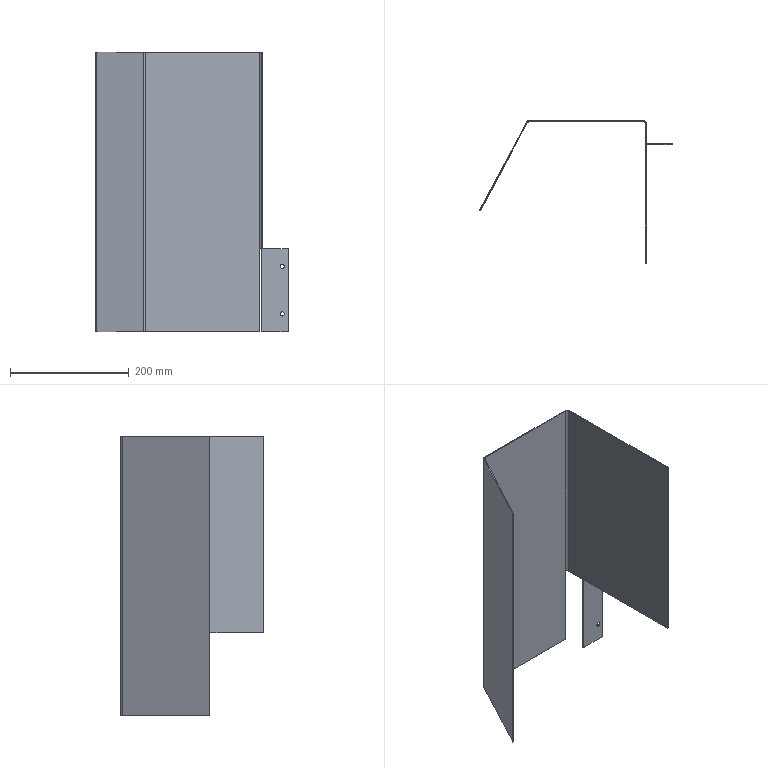Part | SolidWorks | features ICE 4, Extrusion 1, MoveFace 1 | 1 solid | 26 faces | box 323.5 x 240 x 470 mm | volume 385016 mm3 | plane 18 | cylinder 8 | commonest cylinder face diameters 7 x6 10 x2
STEP:
#1=CARTESIAN_POINT('',(313.5,110.,26.5));
#2=VERTEX_POINT('',#1);
#3=CARTESIAN_POINT('',(313.5,110.,33.5));
#4=VERTEX_POINT('',#3);
#5=CARTESIAN_POINT('',(313.5,110.,30.));
#6=DIRECTION('',(0.,1.,0.));
#7=DIRECTION('',(0.,0.,1.));
#8=AXIS2_PLACEMENT_3D('',#5,#6,#7);
#9=CIRCLE('',#8,3.5);
#10=EDGE_CURVE('',#2,#4,#9,.T.);
#11=ORIENTED_EDGE('',*,*,#10,.F.);
#12=CARTESIAN_POINT('',(313.5,111.5,26.5));
#13=VERTEX_POINT('',#12);
#14=CARTESIAN_POINT('',(313.5,110.,26.5));
#15=DIRECTION('',(0.,1.,0.));
#16=VECTOR('',#15,1000.);
#17=LINE('',#14,#16);
#18=EDGE_CURVE('',#2,#13,#17,.T.);
#19=ORIENTED_EDGE('',*,*,#18,.T.);
#20=CARTESIAN_POINT('',(313.5,111.5,33.5));
#21=VERTEX_POINT('',#20);
#22=CARTESIAN_POINT('',(313.5,111.5,30.));
#23=DIRECTION('',(0.,1.,0.));
#24=DIRECTION('',(0.,0.,1.));
#25=AXIS2_PLACEMENT_3D('',#22,#23,#24);
#26=CIRCLE('',#25,3.5);
#27=EDGE_CURVE('',#13,#21,#26,.T.);
#28=ORIENTED_EDGE('',*,*,#27,.T.);
#29=CARTESIAN_POINT('',(313.5,110.,33.5));
#30=DIRECTION('',(0.,1.,0.));
#31=VECTOR('',#30,1000.);
#32=LINE('',#29,#31);
#33=EDGE_CURVE('',#4,#21,#32,.T.);
#34=ORIENTED_EDGE('',*,*,#33,.F.);
#35=EDGE_LOOP('',(#11,#19,#28,#34));
#36=FACE_OUTER_BOUND('',#35,.T.);
#37=CARTESIAN_POINT('',(313.5,110.,30.));
#38=DIRECTION('',(0.,1.,0.));
#39=DIRECTION('',(0.,0.,1.));
#40=AXIS2_PLACEMENT_3D('',#37,#38,#39);
#41=CYLINDRICAL_SURFACE('',#40,3.5);
#42=ADVANCED_FACE('',(#36),#41,.F.);
#43=CARTESIAN_POINT('',(313.5,110.,106.5));
#44=VERTEX_POINT('',#43);
#45=CARTESIAN_POINT('',(313.5,110.,113.5));
#46=VERTEX_POINT('',#45);
#47=CARTESIAN_POINT('',(313.5,110.,110.));
#48=DIRECTION('',(0.,1.,0.));
#49=DIRECTION('',(0.,0.,1.));
#50=AXIS2_PLACEMENT_3D('',#47,#48,#49);
#51=CIRCLE('',#50,3.5);
#52=EDGE_CURVE('',#44,#46,#51,.T.);
#53=ORIENTED_EDGE('',*,*,#52,.F.);
#54=CARTESIAN_POINT('',(313.5,111.5,106.5));
#55=VERTEX_POINT('',#54);
#56=CARTESIAN_POINT('',(313.5,110.,106.5));
#57=DIRECTION('',(0.,1.,0.));
#58=VECTOR('',#57,1000.);
#59=LINE('',#56,#58);
#60=EDGE_CURVE('',#44,#55,#59,.T.);
#61=ORIENTED_EDGE('',*,*,#60,.T.);
#62=CARTESIAN_POINT('',(313.5,111.5,113.5));
#63=VERTEX_POINT('',#62);
#64=CARTESIAN_POINT('',(313.5,111.5,110.));
#65=DIRECTION('',(0.,1.,0.));
#66=DIRECTION('',(0.,0.,1.));
#67=AXIS2_PLACEMENT_3D('',#64,#65,#66);
#68=CIRCLE('',#67,3.5);
#69=EDGE_CURVE('',#55,#63,#68,.T.);
#70=ORIENTED_EDGE('',*,*,#69,.T.);
#71=CARTESIAN_POINT('',(313.5,110.,113.5));
#72=DIRECTION('',(0.,1.,0.));
#73=VECTOR('',#72,1000.);
#74=LINE('',#71,#73);
#75=EDGE_CURVE('',#46,#63,#74,.T.);
#76=ORIENTED_EDGE('',*,*,#75,.F.);
#77=EDGE_LOOP('',(#53,#61,#70,#76));
#78=FACE_OUTER_BOUND('',#77,.T.);
#79=CARTESIAN_POINT('',(313.5,110.,110.));
#80=DIRECTION('',(0.,1.,0.));
#81=DIRECTION('',(0.,0.,1.));
#82=AXIS2_PLACEMENT_3D('',#79,#80,#81);
#83=CYLINDRICAL_SURFACE('',#82,3.5);
#84=ADVANCED_FACE('',(#78),#83,.F.);
#85=CARTESIAN_POINT('',(278.5,110.,140.));
#86=VERTEX_POINT('',#85);
#87=CARTESIAN_POINT('',(278.5,-90.,140.));
#88=VERTEX_POINT('',#87);
#89=CARTESIAN_POINT('',(278.5,145.,140.));
#90=DIRECTION('',(0.,-1.,0.));
#91=VECTOR('',#90,1000.);
#92=LINE('',#89,#91);
#93=EDGE_CURVE('',#86,#88,#92,.T.);
#94=ORIENTED_EDGE('',*,*,#93,.F.);
#95=CARTESIAN_POINT('',(280.,110.,140.));
#96=VERTEX_POINT('',#95);
#97=CARTESIAN_POINT('',(280.,110.,140.));
#98=DIRECTION('',(1.,0.,0.));
#99=VECTOR('',#98,1000.);
#100=LINE('',#97,#99);
#101=EDGE_CURVE('',#86,#96,#100,.T.);
#102=ORIENTED_EDGE('',*,*,#101,.T.);
#103=CARTESIAN_POINT('',(280.,-90.,140.));
#104=VERTEX_POINT('',#103);
#105=CARTESIAN_POINT('',(280.,145.,140.));
#106=DIRECTION('',(0.,-1.,0.));
#107=VECTOR('',#106,1000.);
#108=LINE('',#105,#107);
#109=EDGE_CURVE('',#96,#104,#108,.T.);
#110=ORIENTED_EDGE('',*,*,#109,.T.);
#111=CARTESIAN_POINT('',(280.,-90.,140.));
#112=DIRECTION('',(1.,0.,0.));
#113=VECTOR('',#112,1000.);
#114=LINE('',#111,#113);
#115=EDGE_CURVE('',#88,#104,#114,.T.);
#116=ORIENTED_EDGE('',*,*,#115,.F.);
#117=EDGE_LOOP('',(#94,#102,#110,#116));
#118=FACE_OUTER_BOUND('',#117,.T.);
#119=CARTESIAN_POINT('',(280.,145.,140.));
#120=DIRECTION('',(0.,0.,-1.));
#121=DIRECTION('',(-1.,0.,0.));
#122=AXIS2_PLACEMENT_3D('',#119,#120,#121);
#123=PLANE('',#122);
#124=ADVANCED_FACE('',(#118),#123,.T.);
#125=CARTESIAN_POINT('',(278.5,145.,140.));
#126=VERTEX_POINT('',#125);
#127=CARTESIAN_POINT('',(278.5,111.5,140.));
#128=VERTEX_POINT('',#127);
#129=CARTESIAN_POINT('',(278.5,145.,140.));
#130=DIRECTION('',(0.,-1.,0.));
#131=VECTOR('',#130,1000.);
#132=LINE('',#129,#131);
#133=EDGE_CURVE('',#126,#128,#132,.T.);
#134=ORIENTED_EDGE('',*,*,#133,.T.);
#135=CARTESIAN_POINT('',(278.5,111.5,0.));
#136=VERTEX_POINT('',#135);
#137=CARTESIAN_POINT('',(278.5,111.5,0.));
#138=DIRECTION('',(0.,0.,1.));
#139=VECTOR('',#138,1000.);
#140=LINE('',#137,#139);
#141=EDGE_CURVE('',#136,#128,#140,.T.);
#142=ORIENTED_EDGE('',*,*,#141,.F.);
#143=CARTESIAN_POINT('',(278.5,110.,0.));
#144=VERTEX_POINT('',#143);
#145=CARTESIAN_POINT('',(278.5,111.5,0.));
#146=DIRECTION('',(0.,-1.,0.));
#147=VECTOR('',#146,1000.);
#148=LINE('',#145,#147);
#149=EDGE_CURVE('',#136,#144,#148,.T.);
#150=ORIENTED_EDGE('',*,*,#149,.T.);
#151=CARTESIAN_POINT('',(278.5,110.,0.));
#152=DIRECTION('',(0.,0.,1.));
#153=VECTOR('',#152,1000.);
#154=LINE('',#151,#153);
#155=EDGE_CURVE('',#144,#86,#154,.T.);
#156=ORIENTED_EDGE('',*,*,#155,.T.);
#157=ORIENTED_EDGE('',*,*,#93,.T.);
#158=CARTESIAN_POINT('',(278.5,-90.,470.));
#159=VERTEX_POINT('',#158);
#160=CARTESIAN_POINT('',(278.5,-90.,470.));
#161=DIRECTION('',(0.,0.,-1.));
#162=VECTOR('',#161,1000.);
#163=LINE('',#160,#162);
#164=EDGE_CURVE('',#159,#88,#163,.T.);
#165=ORIENTED_EDGE('',*,*,#164,.F.);
#166=CARTESIAN_POINT('',(278.5,145.,470.));
#167=VERTEX_POINT('',#166);
#168=CARTESIAN_POINT('',(278.5,145.,470.));
#169=DIRECTION('',(0.,-1.,0.));
#170=VECTOR('',#169,1000.);
#171=LINE('',#168,#170);
#172=EDGE_CURVE('',#167,#159,#171,.T.);
#173=ORIENTED_EDGE('',*,*,#172,.F.);
#174=CARTESIAN_POINT('',(278.5,145.,470.));
#175=DIRECTION('',(0.,0.,-1.));
#176=VECTOR('',#175,1000.);
#177=LINE('',#174,#176);
#178=EDGE_CURVE('',#167,#126,#177,.T.);
#179=ORIENTED_EDGE('',*,*,#178,.T.);
#180=EDGE_LOOP('',(#134,#142,#150,#156,#157,#165,#173,#179));
#181=FACE_OUTER_BOUND('',#180,.T.);
#182=CARTESIAN_POINT('',(278.5,145.,470.));
#183=DIRECTION('',(1.,0.,0.));
#184=DIRECTION('',(0.,1.,0.));
#185=AXIS2_PLACEMENT_3D('',#182,#183,#184);
#186=PLANE('',#185);
#187=ADVANCED_FACE('',(#181),#186,.F.);
#188=ORIENTED_EDGE('',*,*,#164,.T.);
#189=ORIENTED_EDGE('',*,*,#115,.T.);
#190=CARTESIAN_POINT('',(280.,-90.,470.));
#191=VERTEX_POINT('',#190);
#192=CARTESIAN_POINT('',(280.,-90.,470.));
#193=DIRECTION('',(0.,0.,-1.));
#194=VECTOR('',#193,1000.);
#195=LINE('',#192,#194);
#196=EDGE_CURVE('',#191,#104,#195,.T.);
#197=ORIENTED_EDGE('',*,*,#196,.F.);
#198=CARTESIAN_POINT('',(280.,-90.,470.));
#199=DIRECTION('',(-1.,0.,0.));
#200=VECTOR('',#199,1000.);
#201=LINE('',#198,#200);
#202=EDGE_CURVE('',#191,#159,#201,.T.);
#203=ORIENTED_EDGE('',*,*,#202,.T.);
#204=EDGE_LOOP('',(#188,#189,#197,#203));
#205=FACE_OUTER_BOUND('',#204,.T.);
#206=CARTESIAN_POINT('',(280.,-90.,470.));
#207=DIRECTION('',(0.,-1.,0.));
#208=DIRECTION('',(0.,0.,-1.));
#209=AXIS2_PLACEMENT_3D('',#206,#207,#208);
#210=PLANE('',#209);
#211=ADVANCED_FACE('',(#205),#210,.T.);
#212=ORIENTED_EDGE('',*,*,#196,.T.);
#213=ORIENTED_EDGE('',*,*,#109,.F.);
#214=CARTESIAN_POINT('',(280.,111.5,140.));
#215=VERTEX_POINT('',#214);
#216=CARTESIAN_POINT('',(280.,145.,140.));
#217=DIRECTION('',(0.,-1.,0.));
#218=VECTOR('',#217,1000.);
#219=LINE('',#216,#218);
#220=EDGE_CURVE('',#215,#96,#219,.T.);
#221=ORIENTED_EDGE('',*,*,#220,.F.);
#222=CARTESIAN_POINT('',(280.,145.,140.));
#223=VERTEX_POINT('',#222);
#224=CARTESIAN_POINT('',(280.,145.,140.));
#225=DIRECTION('',(0.,-1.,0.));
#226=VECTOR('',#225,1000.);
#227=LINE('',#224,#226);
#228=EDGE_CURVE('',#223,#215,#227,.T.);
#229=ORIENTED_EDGE('',*,*,#228,.F.);
#230=CARTESIAN_POINT('',(280.,145.,470.));
#231=VERTEX_POINT('',#230);
#232=CARTESIAN_POINT('',(280.,145.,470.));
#233=DIRECTION('',(0.,0.,-1.));
#234=VECTOR('',#233,1000.);
#235=LINE('',#232,#234);
#236=EDGE_CURVE('',#231,#223,#235,.T.);
#237=ORIENTED_EDGE('',*,*,#236,.F.);
#238=CARTESIAN_POINT('',(280.,145.,470.));
#239=DIRECTION('',(0.,-1.,0.));
#240=VECTOR('',#239,1000.);
#241=LINE('',#238,#240);
#242=EDGE_CURVE('',#231,#191,#241,.T.);
#243=ORIENTED_EDGE('',*,*,#242,.T.);
#244=EDGE_LOOP('',(#212,#213,#221,#229,#237,#243));
#245=FACE_OUTER_BOUND('',#244,.T.);
#246=CARTESIAN_POINT('',(280.,145.,470.));
#247=DIRECTION('',(1.,0.,0.));
#248=DIRECTION('',(0.,1.,0.));
#249=AXIS2_PLACEMENT_3D('',#246,#247,#248);
#250=PLANE('',#249);
#251=ADVANCED_FACE('',(#245),#250,.T.);
#252=CARTESIAN_POINT('',(275.,148.5,0.));
#253=VERTEX_POINT('',#252);
#254=CARTESIAN_POINT('',(275.,150.,0.));
#255=VERTEX_POINT('',#254);
#256=CARTESIAN_POINT('',(275.,91.5,0.));
#257=DIRECTION('',(0.,1.,0.));
#258=VECTOR('',#257,1000.);
#259=LINE('',#256,#258);
#260=EDGE_CURVE('',#253,#255,#259,.T.);
#261=ORIENTED_EDGE('',*,*,#260,.F.);
#262=CARTESIAN_POINT('',(83.,148.5,0.));
#263=VERTEX_POINT('',#262);
#264=CARTESIAN_POINT('',(83.,148.5,0.));
#265=DIRECTION('',(1.,0.,0.));
#266=VECTOR('',#265,1000.);
#267=LINE('',#264,#266);
#268=EDGE_CURVE('',#263,#253,#267,.T.);
#269=ORIENTED_EDGE('',*,*,#268,.F.);
#270=CARTESIAN_POINT('',(79.912,146.647,0.));
#271=VERTEX_POINT('',#270);
#272=CARTESIAN_POINT('',(83.,145.,0.));
#273=DIRECTION('',(0.,0.,-1.));
#274=DIRECTION('',(-1.,0.,0.));
#275=AXIS2_PLACEMENT_3D('',#272,#273,#274);
#276=CIRCLE('',#275,3.5);
#277=EDGE_CURVE('',#271,#263,#276,.T.);
#278=ORIENTED_EDGE('',*,*,#277,.F.);
#279=CARTESIAN_POINT('',(1.7,0.,0.));
#280=VERTEX_POINT('',#279);
#281=CARTESIAN_POINT('',(1.7,0.,0.));
#282=DIRECTION('',(0.4706,0.8824,0.));
#283=VECTOR('',#282,1000.);
#284=LINE('',#281,#283);
#285=EDGE_CURVE('',#280,#271,#284,.T.);
#286=ORIENTED_EDGE('',*,*,#285,.F.);
#287=CARTESIAN_POINT('',(0.,0.,0.));
#288=VERTEX_POINT('',#287);
#289=CARTESIAN_POINT('',(0.,0.,0.));
#290=DIRECTION('',(1.,0.,0.));
#291=VECTOR('',#290,1000.);
#292=LINE('',#289,#291);
#293=EDGE_CURVE('',#288,#280,#292,.T.);
#294=ORIENTED_EDGE('',*,*,#293,.F.);
#295=CARTESIAN_POINT('',(78.588,147.353,0.));
#296=VERTEX_POINT('',#295);
#297=CARTESIAN_POINT('',(0.,0.,0.));
#298=DIRECTION('',(0.4706,0.8824,0.));
#299=VECTOR('',#298,1000.);
#300=LINE('',#297,#299);
#301=EDGE_CURVE('',#288,#296,#300,.T.);
#302=ORIENTED_EDGE('',*,*,#301,.T.);
#303=CARTESIAN_POINT('',(83.,150.,0.));
#304=VERTEX_POINT('',#303);
#305=CARTESIAN_POINT('',(83.,145.,0.));
#306=DIRECTION('',(0.,0.,-1.));
#307=DIRECTION('',(-1.,0.,0.));
#308=AXIS2_PLACEMENT_3D('',#305,#306,#307);
#309=CIRCLE('',#308,5.);
#310=EDGE_CURVE('',#296,#304,#309,.T.);
#311=ORIENTED_EDGE('',*,*,#310,.T.);
#312=CARTESIAN_POINT('',(83.,150.,0.));
#313=DIRECTION('',(1.,0.,0.));
#314=VECTOR('',#313,1000.);
#315=LINE('',#312,#314);
#316=EDGE_CURVE('',#304,#255,#315,.T.);
#317=ORIENTED_EDGE('',*,*,#316,.T.);
#318=EDGE_LOOP('',(#261,#269,#278,#286,#294,#302,#311,#317));
#319=FACE_OUTER_BOUND('',#318,.T.);
#320=CARTESIAN_POINT('',(83.,145.,0.));
#321=DIRECTION('',(0.,0.,-1.));
#322=DIRECTION('',(-1.,0.,0.));
#323=AXIS2_PLACEMENT_3D('',#320,#321,#322);
#324=PLANE('',#323);
#325=ADVANCED_FACE('',(#319),#324,.T.);
#326=ORIENTED_EDGE('',*,*,#293,.T.);
#327=CARTESIAN_POINT('',(1.7,0.,470.));
#328=VERTEX_POINT('',#327);
#329=CARTESIAN_POINT('',(1.7,0.,470.));
#330=DIRECTION('',(0.,0.,-1.));
#331=VECTOR('',#330,1000.);
#332=LINE('',#329,#331);
#333=EDGE_CURVE('',#328,#280,#332,.T.);
#334=ORIENTED_EDGE('',*,*,#333,.F.);
#335=CARTESIAN_POINT('',(0.,0.,470.));
#336=VERTEX_POINT('',#335);
#337=CARTESIAN_POINT('',(0.,0.,470.));
#338=DIRECTION('',(1.,0.,0.));
#339=VECTOR('',#338,1000.);
#340=LINE('',#337,#339);
#341=EDGE_CURVE('',#336,#328,#340,.T.);
#342=ORIENTED_EDGE('',*,*,#341,.F.);
#343=CARTESIAN_POINT('',(0.,0.,470.));
#344=DIRECTION('',(0.,0.,-1.));
#345=VECTOR('',#344,1000.);
#346=LINE('',#343,#345);
#347=EDGE_CURVE('',#336,#288,#346,.T.);
#348=ORIENTED_EDGE('',*,*,#347,.T.);
#349=EDGE_LOOP('',(#326,#334,#342,#348));
#350=FACE_OUTER_BOUND('',#349,.T.);
#351=CARTESIAN_POINT('',(0.,0.,470.));
#352=DIRECTION('',(0.,1.,0.));
#353=DIRECTION('',(0.,0.,1.));
#354=AXIS2_PLACEMENT_3D('',#351,#352,#353);
#355=PLANE('',#354);
#356=ADVANCED_FACE('',(#350),#355,.F.);
#357=ORIENTED_EDGE('',*,*,#285,.T.);
#358=CARTESIAN_POINT('',(79.912,146.647,470.));
#359=VERTEX_POINT('',#358);
#360=CARTESIAN_POINT('',(79.912,146.647,470.));
#361=DIRECTION('',(0.,0.,-1.));
#362=VECTOR('',#361,1000.);
#363=LINE('',#360,#362);
#364=EDGE_CURVE('',#359,#271,#363,.T.);
#365=ORIENTED_EDGE('',*,*,#364,.F.);
#366=CARTESIAN_POINT('',(1.7,0.,470.));
#367=DIRECTION('',(0.4706,0.8824,0.));
#368=VECTOR('',#367,1000.);
#369=LINE('',#366,#368);
#370=EDGE_CURVE('',#328,#359,#369,.T.);
#371=ORIENTED_EDGE('',*,*,#370,.F.);
#372=ORIENTED_EDGE('',*,*,#333,.T.);
#373=EDGE_LOOP('',(#357,#365,#371,#372));
#374=FACE_OUTER_BOUND('',#373,.T.);
#375=CARTESIAN_POINT('',(1.7,0.,470.));
#376=DIRECTION('',(-0.8824,0.4706,0.));
#377=DIRECTION('',(-0.4706,-0.8824,0.));
#378=AXIS2_PLACEMENT_3D('',#375,#376,#377);
#379=PLANE('',#378);
#380=ADVANCED_FACE('',(#374),#379,.F.);
#381=ORIENTED_EDGE('',*,*,#277,.T.);
#382=CARTESIAN_POINT('',(83.,148.5,470.));
#383=VERTEX_POINT('',#382);
#384=CARTESIAN_POINT('',(83.,148.5,470.));
#385=DIRECTION('',(0.,0.,-1.));
#386=VECTOR('',#385,1000.);
#387=LINE('',#384,#386);
#388=EDGE_CURVE('',#383,#263,#387,.T.);
#389=ORIENTED_EDGE('',*,*,#388,.F.);
#390=CARTESIAN_POINT('',(83.,145.,470.));
#391=DIRECTION('',(0.,0.,-1.));
#392=DIRECTION('',(-1.,0.,0.));
#393=AXIS2_PLACEMENT_3D('',#390,#391,#392);
#394=CIRCLE('',#393,3.5);
#395=EDGE_CURVE('',#359,#383,#394,.T.);
#396=ORIENTED_EDGE('',*,*,#395,.F.);
#397=ORIENTED_EDGE('',*,*,#364,.T.);
#398=EDGE_LOOP('',(#381,#389,#396,#397));
#399=FACE_OUTER_BOUND('',#398,.T.);
#400=CARTESIAN_POINT('',(83.,145.,470.));
#401=DIRECTION('',(0.,0.,-1.));
#402=DIRECTION('',(-1.,0.,0.));
#403=AXIS2_PLACEMENT_3D('',#400,#401,#402);
#404=CYLINDRICAL_SURFACE('',#403,3.5);
#405=ADVANCED_FACE('',(#399),#404,.F.);
#406=ORIENTED_EDGE('',*,*,#268,.T.);
#407=CARTESIAN_POINT('',(275.,148.5,140.));
#408=VERTEX_POINT('',#407);
#409=CARTESIAN_POINT('',(275.,148.5,470.));
#410=DIRECTION('',(0.,0.,-1.));
#411=VECTOR('',#410,1000.);
#412=LINE('',#409,#411);
#413=EDGE_CURVE('',#408,#253,#412,.T.);
#414=ORIENTED_EDGE('',*,*,#413,.F.);
#415=CARTESIAN_POINT('',(275.,148.5,470.));
#416=VERTEX_POINT('',#415);
#417=CARTESIAN_POINT('',(275.,148.5,470.));
#418=DIRECTION('',(0.,0.,-1.));
#419=VECTOR('',#418,1000.);
#420=LINE('',#417,#419);
#421=EDGE_CURVE('',#416,#408,#420,.T.);
#422=ORIENTED_EDGE('',*,*,#421,.F.);
#423=CARTESIAN_POINT('',(83.,148.5,470.));
#424=DIRECTION('',(1.,0.,0.));
#425=VECTOR('',#424,1000.);
#426=LINE('',#423,#425);
#427=EDGE_CURVE('',#383,#416,#426,.T.);
#428=ORIENTED_EDGE('',*,*,#427,.F.);
#429=ORIENTED_EDGE('',*,*,#388,.T.);
#430=EDGE_LOOP('',(#406,#414,#422,#428,#429));
#431=FACE_OUTER_BOUND('',#430,.T.);
#432=CARTESIAN_POINT('',(83.,148.5,470.));
#433=DIRECTION('',(0.,1.,0.));
#434=DIRECTION('',(0.,0.,1.));
#435=AXIS2_PLACEMENT_3D('',#432,#433,#434);
#436=PLANE('',#435);
#437=ADVANCED_FACE('',(#431),#436,.F.);
#438=CARTESIAN_POINT('',(275.,145.,140.));
#439=DIRECTION('',(0.,0.,1.));
#440=DIRECTION('',(1.,0.,0.));
#441=AXIS2_PLACEMENT_3D('',#438,#439,#440);
#442=CIRCLE('',#441,3.5);
#443=EDGE_CURVE('',#126,#408,#442,.T.);
#444=ORIENTED_EDGE('',*,*,#443,.F.);
#445=ORIENTED_EDGE('',*,*,#178,.F.);
#446=CARTESIAN_POINT('',(275.,145.,470.));
#447=DIRECTION('',(0.,0.,1.));
#448=DIRECTION('',(1.,0.,0.));
#449=AXIS2_PLACEMENT_3D('',#446,#447,#448);
#450=CIRCLE('',#449,3.5);
#451=EDGE_CURVE('',#167,#416,#450,.T.);
#452=ORIENTED_EDGE('',*,*,#451,.T.);
#453=ORIENTED_EDGE('',*,*,#421,.T.);
#454=EDGE_LOOP('',(#444,#445,#452,#453));
#455=FACE_OUTER_BOUND('',#454,.T.);
#456=CARTESIAN_POINT('',(275.,145.,470.));
#457=DIRECTION('',(0.,0.,-1.));
#458=DIRECTION('',(-1.,0.,0.));
#459=AXIS2_PLACEMENT_3D('',#456,#457,#458);
#460=CYLINDRICAL_SURFACE('',#459,3.5);
#461=ADVANCED_FACE('',(#455),#460,.F.);
#462=ORIENTED_EDGE('',*,*,#236,.T.);
#463=CARTESIAN_POINT('',(275.,150.,140.));
#464=VERTEX_POINT('',#463);
#465=CARTESIAN_POINT('',(275.,145.,140.));
#466=DIRECTION('',(0.,0.,1.));
#467=DIRECTION('',(1.,0.,0.));
#468=AXIS2_PLACEMENT_3D('',#465,#466,#467);
#469=CIRCLE('',#468,5.);
#470=EDGE_CURVE('',#223,#464,#469,.T.);
#471=ORIENTED_EDGE('',*,*,#470,.T.);
#472=CARTESIAN_POINT('',(275.,150.,470.));
#473=VERTEX_POINT('',#472);
#474=CARTESIAN_POINT('',(275.,150.,470.));
#475=DIRECTION('',(0.,0.,-1.));
#476=VECTOR('',#475,1000.);
#477=LINE('',#474,#476);
#478=EDGE_CURVE('',#473,#464,#477,.T.);
#479=ORIENTED_EDGE('',*,*,#478,.F.);
#480=CARTESIAN_POINT('',(275.,145.,470.));
#481=DIRECTION('',(0.,0.,1.));
#482=DIRECTION('',(1.,0.,0.));
#483=AXIS2_PLACEMENT_3D('',#480,#481,#482);
#484=CIRCLE('',#483,5.);
#485=EDGE_CURVE('',#231,#473,#484,.T.);
#486=ORIENTED_EDGE('',*,*,#485,.F.);
#487=EDGE_LOOP('',(#462,#471,#479,#486));
#488=FACE_OUTER_BOUND('',#487,.T.);
#489=CARTESIAN_POINT('',(275.,145.,470.));
#490=DIRECTION('',(0.,0.,-1.));
#491=DIRECTION('',(-1.,0.,0.));
#492=AXIS2_PLACEMENT_3D('',#489,#490,#491);
#493=CYLINDRICAL_SURFACE('',#492,5.);
#494=ADVANCED_FACE('',(#488),#493,.T.);
#495=ORIENTED_EDGE('',*,*,#316,.F.);
#496=CARTESIAN_POINT('',(83.,150.,470.));
#497=VERTEX_POINT('',#496);
#498=CARTESIAN_POINT('',(83.,150.,470.));
#499=DIRECTION('',(0.,0.,-1.));
#500=VECTOR('',#499,1000.);
#501=LINE('',#498,#500);
#502=EDGE_CURVE('',#497,#304,#501,.T.);
#503=ORIENTED_EDGE('',*,*,#502,.F.);
#504=CARTESIAN_POINT('',(83.,150.,470.));
#505=DIRECTION('',(1.,0.,0.));
#506=VECTOR('',#505,1000.);
#507=LINE('',#504,#506);
#508=EDGE_CURVE('',#497,#473,#507,.T.);
#509=ORIENTED_EDGE('',*,*,#508,.T.);
#510=ORIENTED_EDGE('',*,*,#478,.T.);
#511=CARTESIAN_POINT('',(275.,150.,0.));
#512=DIRECTION('',(0.,0.,1.));
#513=VECTOR('',#512,1000.);
#514=LINE('',#511,#513);
#515=EDGE_CURVE('',#255,#464,#514,.T.);
#516=ORIENTED_EDGE('',*,*,#515,.F.);
#517=EDGE_LOOP('',(#495,#503,#509,#510,#516));
#518=FACE_OUTER_BOUND('',#517,.T.);
#519=CARTESIAN_POINT('',(83.,150.,470.));
#520=DIRECTION('',(0.,1.,0.));
#521=DIRECTION('',(0.,0.,1.));
#522=AXIS2_PLACEMENT_3D('',#519,#520,#521);
#523=PLANE('',#522);
#524=ADVANCED_FACE('',(#518),#523,.T.);
#525=ORIENTED_EDGE('',*,*,#310,.F.);
#526=CARTESIAN_POINT('',(78.588,147.353,470.));
#527=VERTEX_POINT('',#526);
#528=CARTESIAN_POINT('',(78.588,147.353,470.));
#529=DIRECTION('',(0.,0.,-1.));
#530=VECTOR('',#529,1000.);
#531=LINE('',#528,#530);
#532=EDGE_CURVE('',#527,#296,#531,.T.);
#533=ORIENTED_EDGE('',*,*,#532,.F.);
#534=CARTESIAN_POINT('',(83.,145.,470.));
#535=DIRECTION('',(0.,0.,-1.));
#536=DIRECTION('',(-1.,0.,0.));
#537=AXIS2_PLACEMENT_3D('',#534,#535,#536);
#538=CIRCLE('',#537,5.);
#539=EDGE_CURVE('',#527,#497,#538,.T.);
#540=ORIENTED_EDGE('',*,*,#539,.T.);
#541=ORIENTED_EDGE('',*,*,#502,.T.);
#542=EDGE_LOOP('',(#525,#533,#540,#541));
#543=FACE_OUTER_BOUND('',#542,.T.);
#544=CARTESIAN_POINT('',(83.,145.,470.));
#545=DIRECTION('',(0.,0.,-1.));
#546=DIRECTION('',(-1.,0.,0.));
#547=AXIS2_PLACEMENT_3D('',#544,#545,#546);
#548=CYLINDRICAL_SURFACE('',#547,5.);
#549=ADVANCED_FACE('',(#543),#548,.T.);
#550=ORIENTED_EDGE('',*,*,#301,.F.);
#551=ORIENTED_EDGE('',*,*,#347,.F.);
#552=CARTESIAN_POINT('',(0.,0.,470.));
#553=DIRECTION('',(0.4706,0.8824,0.));
#554=VECTOR('',#553,1000.);
#555=LINE('',#552,#554);
#556=EDGE_CURVE('',#336,#527,#555,.T.);
#557=ORIENTED_EDGE('',*,*,#556,.T.);
#558=ORIENTED_EDGE('',*,*,#532,.T.);
#559=EDGE_LOOP('',(#550,#551,#557,#558));
#560=FACE_OUTER_BOUND('',#559,.T.);
#561=CARTESIAN_POINT('',(0.,0.,470.));
#562=DIRECTION('',(-0.8824,0.4706,0.));
#563=DIRECTION('',(-0.4706,-0.8824,0.));
#564=AXIS2_PLACEMENT_3D('',#561,#562,#563);
#565=PLANE('',#564);
#566=ADVANCED_FACE('',(#560),#565,.T.);
#567=ORIENTED_EDGE('',*,*,#341,.T.);
#568=ORIENTED_EDGE('',*,*,#370,.T.);
#569=ORIENTED_EDGE('',*,*,#395,.T.);
#570=ORIENTED_EDGE('',*,*,#427,.T.);
#571=ORIENTED_EDGE('',*,*,#451,.F.);
#572=ORIENTED_EDGE('',*,*,#172,.T.);
#573=ORIENTED_EDGE('',*,*,#202,.F.);
#574=ORIENTED_EDGE('',*,*,#242,.F.);
#575=ORIENTED_EDGE('',*,*,#485,.T.);
#576=ORIENTED_EDGE('',*,*,#508,.F.);
#577=ORIENTED_EDGE('',*,*,#539,.F.);
#578=ORIENTED_EDGE('',*,*,#556,.F.);
#579=EDGE_LOOP('',(#567,#568,#569,#570,#571,#572,#573,#574,#575,#576,#577,#578));
#580=FACE_OUTER_BOUND('',#579,.T.);
#581=CARTESIAN_POINT('',(83.,145.,470.));
#582=DIRECTION('',(0.,0.,-1.));
#583=DIRECTION('',(-1.,0.,0.));
#584=AXIS2_PLACEMENT_3D('',#581,#582,#583);
#585=PLANE('',#584);
#586=ADVANCED_FACE('',(#580),#585,.F.);
#587=CARTESIAN_POINT('',(280.,111.5,140.));
#588=DIRECTION('',(1.,0.,0.));
#589=VECTOR('',#588,1000.);
#590=LINE('',#587,#589);
#591=EDGE_CURVE('',#128,#215,#590,.T.);
#592=ORIENTED_EDGE('',*,*,#591,.F.);
#593=ORIENTED_EDGE('',*,*,#133,.F.);
#594=ORIENTED_EDGE('',*,*,#443,.T.);
#595=CARTESIAN_POINT('',(275.,91.5,140.));
#596=DIRECTION('',(0.,1.,0.));
#597=VECTOR('',#596,1000.);
#598=LINE('',#595,#597);
#599=EDGE_CURVE('',#408,#464,#598,.T.);
#600=ORIENTED_EDGE('',*,*,#599,.T.);
#601=ORIENTED_EDGE('',*,*,#470,.F.);
#602=ORIENTED_EDGE('',*,*,#228,.T.);
#603=EDGE_LOOP('',(#592,#593,#594,#600,#601,#602));
#604=FACE_OUTER_BOUND('',#603,.T.);
#605=CARTESIAN_POINT('',(280.,145.,140.));
#606=DIRECTION('',(0.,0.,-1.));
#607=DIRECTION('',(-1.,0.,0.));
#608=AXIS2_PLACEMENT_3D('',#605,#606,#607);
#609=PLANE('',#608);
#610=ADVANCED_FACE('',(#604),#609,.T.);
#611=ORIENTED_EDGE('',*,*,#413,.T.);
#612=ORIENTED_EDGE('',*,*,#260,.T.);
#613=ORIENTED_EDGE('',*,*,#515,.T.);
#614=ORIENTED_EDGE('',*,*,#599,.F.);
#615=EDGE_LOOP('',(#611,#612,#613,#614));
#616=FACE_OUTER_BOUND('',#615,.T.);
#617=CARTESIAN_POINT('',(275.,91.5,0.));
#618=DIRECTION('',(-1.,0.,0.));
#619=DIRECTION('',(0.,0.,1.));
#620=AXIS2_PLACEMENT_3D('',#617,#618,#619);
#621=PLANE('',#620);
#622=ADVANCED_FACE('',(#616),#621,.F.);
#623=ORIENTED_EDGE('',*,*,#220,.T.);
#624=CARTESIAN_POINT('',(323.5,110.,140.));
#625=VERTEX_POINT('',#624);
#626=CARTESIAN_POINT('',(275.,110.,140.));
#627=DIRECTION('',(1.,0.,0.));
#628=VECTOR('',#627,1000.);
#629=LINE('',#626,#628);
#630=EDGE_CURVE('',#96,#625,#629,.T.);
#631=ORIENTED_EDGE('',*,*,#630,.T.);
#632=CARTESIAN_POINT('',(323.5,111.5,140.));
#633=VERTEX_POINT('',#632);
#634=CARTESIAN_POINT('',(323.5,111.5,140.));
#635=DIRECTION('',(0.,-1.,0.));
#636=VECTOR('',#635,1000.);
#637=LINE('',#634,#636);
#638=EDGE_CURVE('',#633,#625,#637,.T.);
#639=ORIENTED_EDGE('',*,*,#638,.F.);
#640=CARTESIAN_POINT('',(275.,111.5,140.));
#641=DIRECTION('',(1.,0.,0.));
#642=VECTOR('',#641,1000.);
#643=LINE('',#640,#642);
#644=EDGE_CURVE('',#215,#633,#643,.T.);
#645=ORIENTED_EDGE('',*,*,#644,.F.);
#646=EDGE_LOOP('',(#623,#631,#639,#645));
#647=FACE_OUTER_BOUND('',#646,.T.);
#648=CARTESIAN_POINT('',(275.,111.5,140.));
#649=DIRECTION('',(0.,0.,-1.));
#650=DIRECTION('',(-1.,0.,0.));
#651=AXIS2_PLACEMENT_3D('',#648,#649,#650);
#652=PLANE('',#651);
#653=ADVANCED_FACE('',(#647),#652,.F.);
#654=CARTESIAN_POINT('',(323.5,110.,0.));
#655=VERTEX_POINT('',#654);
#656=CARTESIAN_POINT('',(323.5,110.,140.));
#657=DIRECTION('',(0.,0.,-1.));
#658=VECTOR('',#657,1000.);
#659=LINE('',#656,#658);
#660=EDGE_CURVE('',#625,#655,#659,.T.);
#661=ORIENTED_EDGE('',*,*,#660,.T.);
#662=CARTESIAN_POINT('',(323.5,111.5,0.));
#663=VERTEX_POINT('',#662);
#664=CARTESIAN_POINT('',(323.5,111.5,0.));
#665=DIRECTION('',(0.,-1.,0.));
#666=VECTOR('',#665,1000.);
#667=LINE('',#664,#666);
#668=EDGE_CURVE('',#663,#655,#667,.T.);
#669=ORIENTED_EDGE('',*,*,#668,.F.);
#670=CARTESIAN_POINT('',(323.5,111.5,140.));
#671=DIRECTION('',(0.,0.,-1.));
#672=VECTOR('',#671,1000.);
#673=LINE('',#670,#672);
#674=EDGE_CURVE('',#633,#663,#673,.T.);
#675=ORIENTED_EDGE('',*,*,#674,.F.);
#676=ORIENTED_EDGE('',*,*,#638,.T.);
#677=EDGE_LOOP('',(#661,#669,#675,#676));
#678=FACE_OUTER_BOUND('',#677,.T.);
#679=CARTESIAN_POINT('',(323.5,111.5,140.));
#680=DIRECTION('',(-1.,0.,0.));
#681=DIRECTION('',(0.,0.,1.));
#682=AXIS2_PLACEMENT_3D('',#679,#680,#681);
#683=PLANE('',#682);
#684=ADVANCED_FACE('',(#678),#683,.F.);
#685=CARTESIAN_POINT('',(323.5,110.,0.));
#686=DIRECTION('',(-1.,0.,0.));
#687=VECTOR('',#686,1000.);
#688=LINE('',#685,#687);
#689=EDGE_CURVE('',#655,#144,#688,.T.);
#690=ORIENTED_EDGE('',*,*,#689,.T.);
#691=ORIENTED_EDGE('',*,*,#149,.F.);
#692=CARTESIAN_POINT('',(323.5,111.5,0.));
#693=DIRECTION('',(-1.,0.,0.));
#694=VECTOR('',#693,1000.);
#695=LINE('',#692,#694);
#696=EDGE_CURVE('',#663,#136,#695,.T.);
#697=ORIENTED_EDGE('',*,*,#696,.F.);
#698=ORIENTED_EDGE('',*,*,#668,.T.);
#699=EDGE_LOOP('',(#690,#691,#697,#698));
#700=FACE_OUTER_BOUND('',#699,.T.);
#701=CARTESIAN_POINT('',(323.5,111.5,0.));
#702=DIRECTION('',(0.,0.,1.));
#703=DIRECTION('',(1.,0.,0.));
#704=AXIS2_PLACEMENT_3D('',#701,#702,#703);
#705=PLANE('',#704);
#706=ADVANCED_FACE('',(#700),#705,.F.);
#707=CARTESIAN_POINT('',(313.5,111.5,30.));
#708=DIRECTION('',(0.,1.,0.));
#709=DIRECTION('',(0.,0.,1.));
#710=AXIS2_PLACEMENT_3D('',#707,#708,#709);
#711=CIRCLE('',#710,3.5);
#712=EDGE_CURVE('',#21,#13,#711,.T.);
#713=ORIENTED_EDGE('',*,*,#712,.F.);
#714=ORIENTED_EDGE('',*,*,#27,.F.);
#715=EDGE_LOOP('',(#713,#714));
#716=FACE_BOUND('',#715,.T.);
#717=CARTESIAN_POINT('',(313.5,111.5,110.));
#718=DIRECTION('',(0.,1.,0.));
#719=DIRECTION('',(0.,0.,1.));
#720=AXIS2_PLACEMENT_3D('',#717,#718,#719);
#721=CIRCLE('',#720,3.5);
#722=EDGE_CURVE('',#63,#55,#721,.T.);
#723=ORIENTED_EDGE('',*,*,#722,.F.);
#724=ORIENTED_EDGE('',*,*,#69,.F.);
#725=EDGE_LOOP('',(#723,#724));
#726=FACE_BOUND('',#725,.T.);
#727=ORIENTED_EDGE('',*,*,#141,.T.);
#728=ORIENTED_EDGE('',*,*,#591,.T.);
#729=ORIENTED_EDGE('',*,*,#644,.T.);
#730=ORIENTED_EDGE('',*,*,#674,.T.);
#731=ORIENTED_EDGE('',*,*,#696,.T.);
#732=EDGE_LOOP('',(#727,#728,#729,#730,#731));
#733=FACE_OUTER_BOUND('',#732,.T.);
#734=CARTESIAN_POINT('',(0.,111.5,0.));
#735=DIRECTION('',(0.,1.,0.));
#736=DIRECTION('',(0.,0.,1.));
#737=AXIS2_PLACEMENT_3D('',#734,#735,#736);
#738=PLANE('',#737);
#739=ADVANCED_FACE('',(#716,#726,#733),#738,.T.);
#740=CARTESIAN_POINT('',(313.5,110.,30.));
#741=DIRECTION('',(0.,1.,0.));
#742=DIRECTION('',(0.,0.,1.));
#743=AXIS2_PLACEMENT_3D('',#740,#741,#742);
#744=CIRCLE('',#743,3.5);
#745=EDGE_CURVE('',#4,#2,#744,.T.);
#746=ORIENTED_EDGE('',*,*,#745,.T.);
#747=ORIENTED_EDGE('',*,*,#10,.T.);
#748=EDGE_LOOP('',(#746,#747));
#749=FACE_BOUND('',#748,.T.);
#750=CARTESIAN_POINT('',(313.5,110.,110.));
#751=DIRECTION('',(0.,1.,0.));
#752=DIRECTION('',(0.,0.,1.));
#753=AXIS2_PLACEMENT_3D('',#750,#751,#752);
#754=CIRCLE('',#753,3.5);
#755=EDGE_CURVE('',#46,#44,#754,.T.);
#756=ORIENTED_EDGE('',*,*,#755,.T.);
#757=ORIENTED_EDGE('',*,*,#52,.T.);
#758=EDGE_LOOP('',(#756,#757));
#759=FACE_BOUND('',#758,.T.);
#760=ORIENTED_EDGE('',*,*,#155,.F.);
#761=ORIENTED_EDGE('',*,*,#689,.F.);
#762=ORIENTED_EDGE('',*,*,#660,.F.);
#763=ORIENTED_EDGE('',*,*,#630,.F.);
#764=ORIENTED_EDGE('',*,*,#101,.F.);
#765=EDGE_LOOP('',(#760,#761,#762,#763,#764));
#766=FACE_OUTER_BOUND('',#765,.T.);
#767=CARTESIAN_POINT('',(0.,110.,0.));
#768=DIRECTION('',(0.,1.,0.));
#769=DIRECTION('',(0.,0.,1.));
#770=AXIS2_PLACEMENT_3D('',#767,#768,#769);
#771=PLANE('',#770);
#772=ADVANCED_FACE('',(#749,#759,#766),#771,.F.);
#773=ORIENTED_EDGE('',*,*,#60,.F.);
#774=ORIENTED_EDGE('',*,*,#755,.F.);
#775=ORIENTED_EDGE('',*,*,#75,.T.);
#776=ORIENTED_EDGE('',*,*,#722,.T.);
#777=EDGE_LOOP('',(#773,#774,#775,#776));
#778=FACE_OUTER_BOUND('',#777,.T.);
#779=CARTESIAN_POINT('',(313.5,110.,110.));
#780=DIRECTION('',(0.,1.,0.));
#781=DIRECTION('',(0.,0.,1.));
#782=AXIS2_PLACEMENT_3D('',#779,#780,#781);
#783=CYLINDRICAL_SURFACE('',#782,3.5);
#784=ADVANCED_FACE('',(#778),#783,.F.);
#785=ORIENTED_EDGE('',*,*,#18,.F.);
#786=ORIENTED_EDGE('',*,*,#745,.F.);
#787=ORIENTED_EDGE('',*,*,#33,.T.);
#788=ORIENTED_EDGE('',*,*,#712,.T.);
#789=EDGE_LOOP('',(#785,#786,#787,#788));
#790=FACE_OUTER_BOUND('',#789,.T.);
#791=CARTESIAN_POINT('',(313.5,110.,30.));
#792=DIRECTION('',(0.,1.,0.));
#793=DIRECTION('',(0.,0.,1.));
#794=AXIS2_PLACEMENT_3D('',#791,#792,#793);
#795=CYLINDRICAL_SURFACE('',#794,3.5);
#796=ADVANCED_FACE('',(#790),#795,.F.);
#797=CLOSED_SHELL('',(#42,#84,#124,#187,#211,#251,#325,#356,#380,#405,#437,#461,#494,#524,#549,#566,#586,#610,#622,#653,#684,#706,#739,#772,#784,#796));
#798=MANIFOLD_SOLID_BREP('',#797);
#799=CARTESIAN_POINT('',(0.,0.,0.));
#800=DIRECTION('',(0.,0.,1.));
#801=DIRECTION('',(1.,0.,0.));
#802=AXIS2_PLACEMENT_3D('',#799,#800,#801);
#803=(LENGTH_UNIT()NAMED_UNIT(*)SI_UNIT(.MILLI.,.METRE.));
#804=UNCERTAINTY_MEASURE_WITH_UNIT(LENGTH_MEASURE(0.00001),#803,'','');
#805=(NAMED_UNIT(*)PLANE_ANGLE_UNIT()SI_UNIT($,.RADIAN.));
#806=(NAMED_UNIT(*)SI_UNIT($,.STERADIAN.)SOLID_ANGLE_UNIT());
#807=(GEOMETRIC_REPRESENTATION_CONTEXT(3)GLOBAL_UNCERTAINTY_ASSIGNED_CONTEXT((#804))GLOBAL_UNIT_ASSIGNED_CONTEXT((#803,#805,#806))REPRESENTATION_CONTEXT('',''));
#808=ADVANCED_BREP_SHAPE_REPRESENTATION('',(#798,#802),#807);